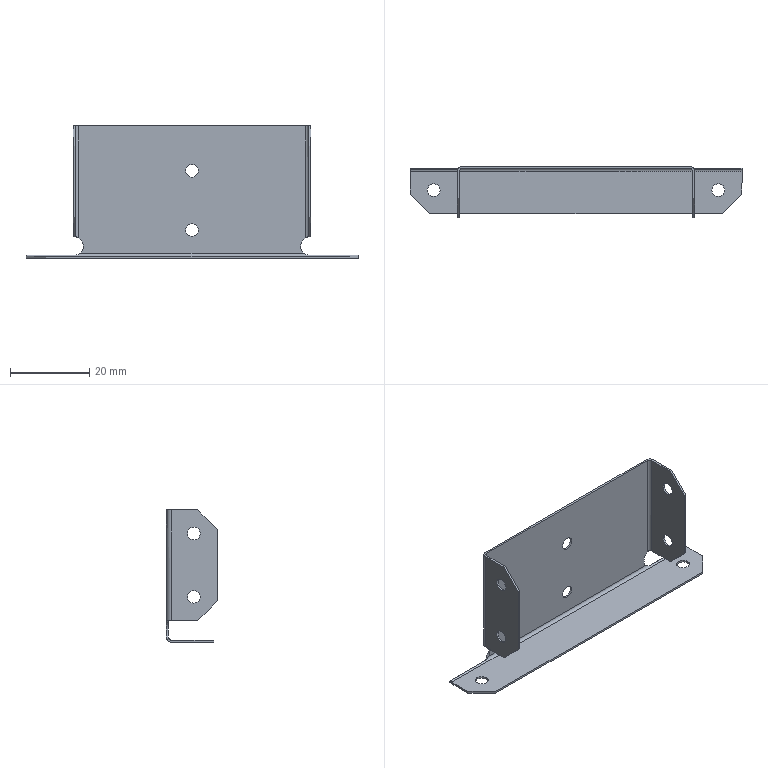Part | SolidWorks | features BaseBody 1 | 1 solid | 52 faces | box 84 x 12.929 x 33.465 mm | volume 1730 mm3 | cylinder 24 | plane 24 | spline 4 | commonest cylinder face diameters 3.2 x16 1.5 x3 2.5 x3 5 x2